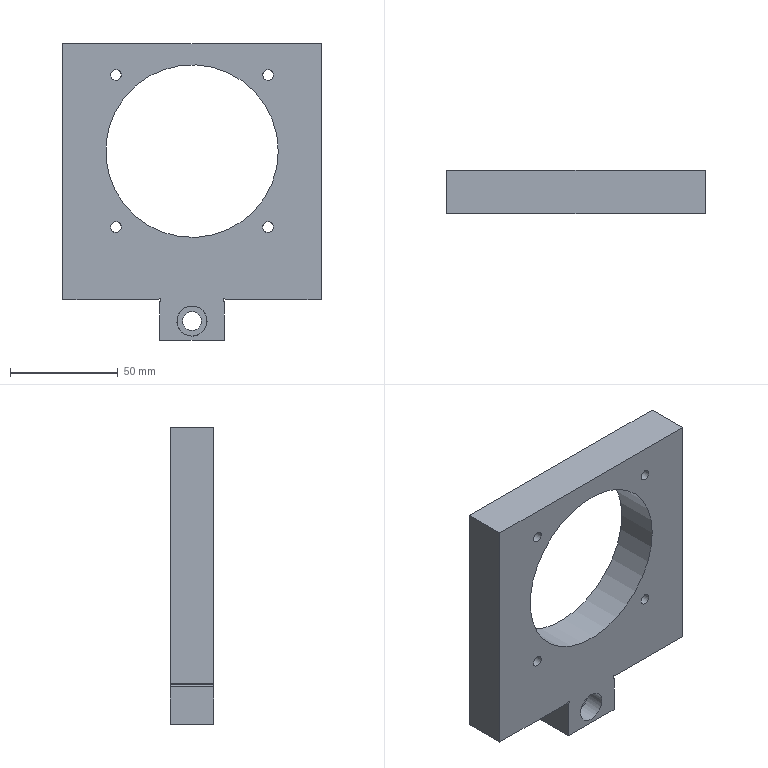Part | STEP file | YBQDJ-PD-3 | 1 solid | 34 faces | box 120 x 20 x 138 mm | volume 191169 mm3 | cylinder 15 | plane 11 | cone 8 | commonest cylinder face diameters 4 x4 5 x4 1 x2 6.8 x2 8.7 x1 14 x1